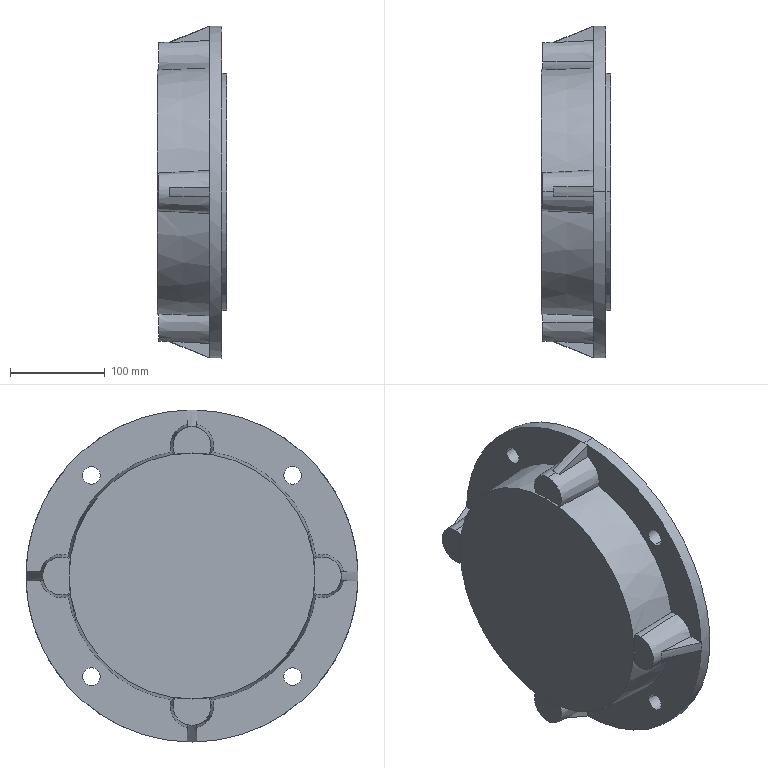Part | STEP file | Input 103 | 1 solid | 62 faces | box 73 x 350 x 350 mm | volume 3966016 mm3 | plane 21 | cone 19 | cylinder 12 | torus 6 | spline 4 | commonest cylinder face diameters 18.5 x8 250 x2 350 x2